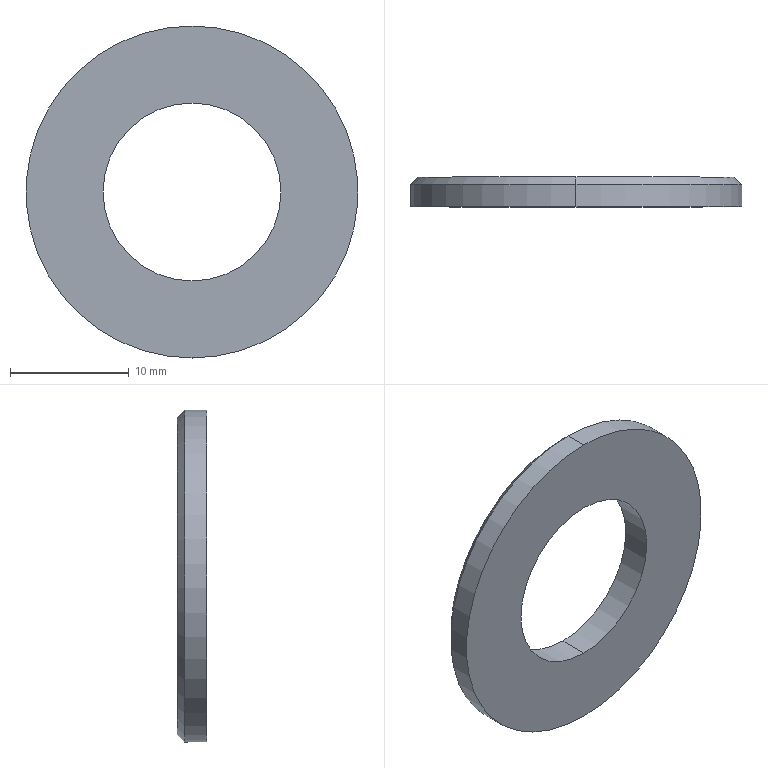Part | SolidWorks | features Revolution 1 | 1 solid | 8 faces | box 28 x 2.5 x 28 mm | volume 1081 mm3 | cylinder 4 | cone 2 | plane 2 | commonest cylinder face diameters 15 x2 28 x2
STEP:
#1=CARTESIAN_POINT('',(0.,10.52,-14.));
#2=VERTEX_POINT('',#1);
#3=CARTESIAN_POINT('',(0.,10.52,14.));
#4=VERTEX_POINT('',#3);
#5=CARTESIAN_POINT('',(0.,10.52,0.));
#6=DIRECTION('',(0.,-1.,0.));
#7=DIRECTION('',(0.,0.,-1.));
#8=AXIS2_PLACEMENT_3D('',#5,#6,#7);
#9=CIRCLE('',#8,14.);
#10=EDGE_CURVE('',#2,#4,#9,.T.);
#11=ORIENTED_EDGE('',*,*,#10,.T.);
#12=CARTESIAN_POINT('',(0.,8.645,14.));
#13=VERTEX_POINT('',#12);
#14=CARTESIAN_POINT('',(0.,0.,14.));
#15=DIRECTION('',(0.,-1.,0.));
#16=VECTOR('',#15,1000.);
#17=LINE('',#14,#16);
#18=EDGE_CURVE('',#4,#13,#17,.T.);
#19=ORIENTED_EDGE('',*,*,#18,.T.);
#20=CARTESIAN_POINT('',(0.,8.645,-14.));
#21=VERTEX_POINT('',#20);
#22=CARTESIAN_POINT('',(0.,8.645,0.));
#23=DIRECTION('',(0.,-1.,0.));
#24=DIRECTION('',(0.,0.,-1.));
#25=AXIS2_PLACEMENT_3D('',#22,#23,#24);
#26=CIRCLE('',#25,14.);
#27=EDGE_CURVE('',#21,#13,#26,.T.);
#28=ORIENTED_EDGE('',*,*,#27,.F.);
#29=CARTESIAN_POINT('',(0.,0.,-14.));
#30=DIRECTION('',(0.,-1.,0.));
#31=VECTOR('',#30,1000.);
#32=LINE('',#29,#31);
#33=EDGE_CURVE('',#2,#21,#32,.T.);
#34=ORIENTED_EDGE('',*,*,#33,.F.);
#35=EDGE_LOOP('',(#11,#19,#28,#34));
#36=FACE_OUTER_BOUND('',#35,.T.);
#37=CARTESIAN_POINT('',(0.,0.,0.));
#38=DIRECTION('',(0.,-1.,0.));
#39=DIRECTION('',(0.,0.,-1.));
#40=AXIS2_PLACEMENT_3D('',#37,#38,#39);
#41=CYLINDRICAL_SURFACE('',#40,14.);
#42=ADVANCED_FACE('',(#36),#41,.T.);
#43=CARTESIAN_POINT('',(0.,11.145,-13.375));
#44=VERTEX_POINT('',#43);
#45=CARTESIAN_POINT('',(0.,11.145,13.375));
#46=VERTEX_POINT('',#45);
#47=CARTESIAN_POINT('',(0.,11.145,0.));
#48=DIRECTION('',(0.,-1.,0.));
#49=DIRECTION('',(0.,0.,-1.));
#50=AXIS2_PLACEMENT_3D('',#47,#48,#49);
#51=CIRCLE('',#50,13.375);
#52=EDGE_CURVE('',#44,#46,#51,.T.);
#53=ORIENTED_EDGE('',*,*,#52,.T.);
#54=CARTESIAN_POINT('',(0.,11.145,13.375));
#55=DIRECTION('',(0.,-0.7071,0.7071));
#56=VECTOR('',#55,1000.);
#57=LINE('',#54,#56);
#58=EDGE_CURVE('',#46,#4,#57,.T.);
#59=ORIENTED_EDGE('',*,*,#58,.T.);
#60=ORIENTED_EDGE('',*,*,#10,.F.);
#61=CARTESIAN_POINT('',(0.,11.145,-13.375));
#62=DIRECTION('',(0.,-0.7071,-0.7071));
#63=VECTOR('',#62,1000.);
#64=LINE('',#61,#63);
#65=EDGE_CURVE('',#44,#2,#64,.T.);
#66=ORIENTED_EDGE('',*,*,#65,.F.);
#67=EDGE_LOOP('',(#53,#59,#60,#66));
#68=FACE_OUTER_BOUND('',#67,.T.);
#69=CARTESIAN_POINT('',(0.,11.145,0.));
#70=DIRECTION('',(0.,-1.,0.));
#71=DIRECTION('',(0.,0.,-1.));
#72=AXIS2_PLACEMENT_3D('',#69,#70,#71);
#73=CONICAL_SURFACE('',#72,13.375,0.7854);
#74=ADVANCED_FACE('',(#68),#73,.T.);
#75=CARTESIAN_POINT('',(0.,11.145,7.5));
#76=VERTEX_POINT('',#75);
#77=CARTESIAN_POINT('',(0.,11.145,-7.5));
#78=VERTEX_POINT('',#77);
#79=CARTESIAN_POINT('',(0.,11.145,0.));
#80=DIRECTION('',(0.,-1.,0.));
#81=DIRECTION('',(0.,0.,-1.));
#82=AXIS2_PLACEMENT_3D('',#79,#80,#81);
#83=CIRCLE('',#82,7.5);
#84=EDGE_CURVE('',#76,#78,#83,.T.);
#85=ORIENTED_EDGE('',*,*,#84,.F.);
#86=CARTESIAN_POINT('',(0.,8.645,7.5));
#87=VERTEX_POINT('',#86);
#88=CARTESIAN_POINT('',(0.,0.,7.5));
#89=DIRECTION('',(0.,-1.,0.));
#90=VECTOR('',#89,1000.);
#91=LINE('',#88,#90);
#92=EDGE_CURVE('',#76,#87,#91,.T.);
#93=ORIENTED_EDGE('',*,*,#92,.T.);
#94=CARTESIAN_POINT('',(0.,8.645,-7.5));
#95=VERTEX_POINT('',#94);
#96=CARTESIAN_POINT('',(0.,8.645,0.));
#97=DIRECTION('',(0.,-1.,0.));
#98=DIRECTION('',(0.,0.,-1.));
#99=AXIS2_PLACEMENT_3D('',#96,#97,#98);
#100=CIRCLE('',#99,7.5);
#101=EDGE_CURVE('',#87,#95,#100,.T.);
#102=ORIENTED_EDGE('',*,*,#101,.T.);
#103=CARTESIAN_POINT('',(0.,0.,-7.5));
#104=DIRECTION('',(0.,-1.,0.));
#105=VECTOR('',#104,1000.);
#106=LINE('',#103,#105);
#107=EDGE_CURVE('',#78,#95,#106,.T.);
#108=ORIENTED_EDGE('',*,*,#107,.F.);
#109=EDGE_LOOP('',(#85,#93,#102,#108));
#110=FACE_OUTER_BOUND('',#109,.T.);
#111=CARTESIAN_POINT('',(0.,0.,0.));
#112=DIRECTION('',(0.,-1.,0.));
#113=DIRECTION('',(0.,0.,-1.));
#114=AXIS2_PLACEMENT_3D('',#111,#112,#113);
#115=CYLINDRICAL_SURFACE('',#114,7.5);
#116=ADVANCED_FACE('',(#110),#115,.F.);
#117=ORIENTED_EDGE('',*,*,#92,.F.);
#118=CARTESIAN_POINT('',(0.,11.145,0.));
#119=DIRECTION('',(0.,-1.,0.));
#120=DIRECTION('',(0.,0.,-1.));
#121=AXIS2_PLACEMENT_3D('',#118,#119,#120);
#122=CIRCLE('',#121,7.5);
#123=EDGE_CURVE('',#78,#76,#122,.T.);
#124=ORIENTED_EDGE('',*,*,#123,.F.);
#125=ORIENTED_EDGE('',*,*,#107,.T.);
#126=CARTESIAN_POINT('',(0.,8.645,0.));
#127=DIRECTION('',(0.,-1.,0.));
#128=DIRECTION('',(0.,0.,-1.));
#129=AXIS2_PLACEMENT_3D('',#126,#127,#128);
#130=CIRCLE('',#129,7.5);
#131=EDGE_CURVE('',#95,#87,#130,.T.);
#132=ORIENTED_EDGE('',*,*,#131,.T.);
#133=EDGE_LOOP('',(#117,#124,#125,#132));
#134=FACE_OUTER_BOUND('',#133,.T.);
#135=CARTESIAN_POINT('',(0.,0.,0.));
#136=DIRECTION('',(0.,-1.,0.));
#137=DIRECTION('',(0.,0.,-1.));
#138=AXIS2_PLACEMENT_3D('',#135,#136,#137);
#139=CYLINDRICAL_SURFACE('',#138,7.5);
#140=ADVANCED_FACE('',(#134),#139,.F.);
#141=ORIENTED_EDGE('',*,*,#52,.F.);
#142=CARTESIAN_POINT('',(0.,11.145,0.));
#143=DIRECTION('',(0.,-1.,0.));
#144=DIRECTION('',(0.,0.,-1.));
#145=AXIS2_PLACEMENT_3D('',#142,#143,#144);
#146=CIRCLE('',#145,13.375);
#147=EDGE_CURVE('',#46,#44,#146,.T.);
#148=ORIENTED_EDGE('',*,*,#147,.F.);
#149=EDGE_LOOP('',(#141,#148));
#150=FACE_OUTER_BOUND('',#149,.T.);
#151=ORIENTED_EDGE('',*,*,#123,.T.);
#152=ORIENTED_EDGE('',*,*,#84,.T.);
#153=EDGE_LOOP('',(#151,#152));
#154=FACE_BOUND('',#153,.T.);
#155=CARTESIAN_POINT('',(-7.5,11.145,0.));
#156=DIRECTION('',(0.,-1.,0.));
#157=DIRECTION('',(0.,0.,-1.));
#158=AXIS2_PLACEMENT_3D('',#155,#156,#157);
#159=PLANE('',#158);
#160=ADVANCED_FACE('',(#150,#154),#159,.F.);
#161=ORIENTED_EDGE('',*,*,#58,.F.);
#162=ORIENTED_EDGE('',*,*,#147,.T.);
#163=ORIENTED_EDGE('',*,*,#65,.T.);
#164=CARTESIAN_POINT('',(0.,10.52,0.));
#165=DIRECTION('',(0.,-1.,0.));
#166=DIRECTION('',(0.,0.,-1.));
#167=AXIS2_PLACEMENT_3D('',#164,#165,#166);
#168=CIRCLE('',#167,14.);
#169=EDGE_CURVE('',#4,#2,#168,.T.);
#170=ORIENTED_EDGE('',*,*,#169,.F.);
#171=EDGE_LOOP('',(#161,#162,#163,#170));
#172=FACE_OUTER_BOUND('',#171,.T.);
#173=CARTESIAN_POINT('',(0.,11.145,0.));
#174=DIRECTION('',(0.,-1.,0.));
#175=DIRECTION('',(0.,0.,-1.));
#176=AXIS2_PLACEMENT_3D('',#173,#174,#175);
#177=CONICAL_SURFACE('',#176,13.375,0.7854);
#178=ADVANCED_FACE('',(#172),#177,.T.);
#179=ORIENTED_EDGE('',*,*,#18,.F.);
#180=ORIENTED_EDGE('',*,*,#169,.T.);
#181=ORIENTED_EDGE('',*,*,#33,.T.);
#182=CARTESIAN_POINT('',(0.,8.645,0.));
#183=DIRECTION('',(0.,-1.,0.));
#184=DIRECTION('',(0.,0.,-1.));
#185=AXIS2_PLACEMENT_3D('',#182,#183,#184);
#186=CIRCLE('',#185,14.);
#187=EDGE_CURVE('',#13,#21,#186,.T.);
#188=ORIENTED_EDGE('',*,*,#187,.F.);
#189=EDGE_LOOP('',(#179,#180,#181,#188));
#190=FACE_OUTER_BOUND('',#189,.T.);
#191=CARTESIAN_POINT('',(0.,0.,0.));
#192=DIRECTION('',(0.,-1.,0.));
#193=DIRECTION('',(0.,0.,-1.));
#194=AXIS2_PLACEMENT_3D('',#191,#192,#193);
#195=CYLINDRICAL_SURFACE('',#194,14.);
#196=ADVANCED_FACE('',(#190),#195,.T.);
#197=ORIENTED_EDGE('',*,*,#131,.F.);
#198=ORIENTED_EDGE('',*,*,#101,.F.);
#199=EDGE_LOOP('',(#197,#198));
#200=FACE_BOUND('',#199,.T.);
#201=ORIENTED_EDGE('',*,*,#27,.T.);
#202=ORIENTED_EDGE('',*,*,#187,.T.);
#203=EDGE_LOOP('',(#201,#202));
#204=FACE_OUTER_BOUND('',#203,.T.);
#205=CARTESIAN_POINT('',(-7.5,8.645,0.));
#206=DIRECTION('',(0.,1.,0.));
#207=DIRECTION('',(0.,0.,1.));
#208=AXIS2_PLACEMENT_3D('',#205,#206,#207);
#209=PLANE('',#208);
#210=ADVANCED_FACE('',(#200,#204),#209,.F.);
#211=CLOSED_SHELL('',(#42,#74,#116,#140,#160,#178,#196,#210));
#212=MANIFOLD_SOLID_BREP('',#211);
#213=CARTESIAN_POINT('',(0.,0.,0.));
#214=DIRECTION('',(0.,0.,1.));
#215=DIRECTION('',(1.,0.,0.));
#216=AXIS2_PLACEMENT_3D('',#213,#214,#215);
#217=(LENGTH_UNIT()NAMED_UNIT(*)SI_UNIT(.MILLI.,.METRE.));
#218=UNCERTAINTY_MEASURE_WITH_UNIT(LENGTH_MEASURE(0.00001),#217,'','');
#219=(NAMED_UNIT(*)PLANE_ANGLE_UNIT()SI_UNIT($,.RADIAN.));
#220=(NAMED_UNIT(*)SI_UNIT($,.STERADIAN.)SOLID_ANGLE_UNIT());
#221=(GEOMETRIC_REPRESENTATION_CONTEXT(3)GLOBAL_UNCERTAINTY_ASSIGNED_CONTEXT((#218))GLOBAL_UNIT_ASSIGNED_CONTEXT((#217,#219,#220))REPRESENTATION_CONTEXT('',''));
#222=ADVANCED_BREP_SHAPE_REPRESENTATION('',(#212,#216),#221);